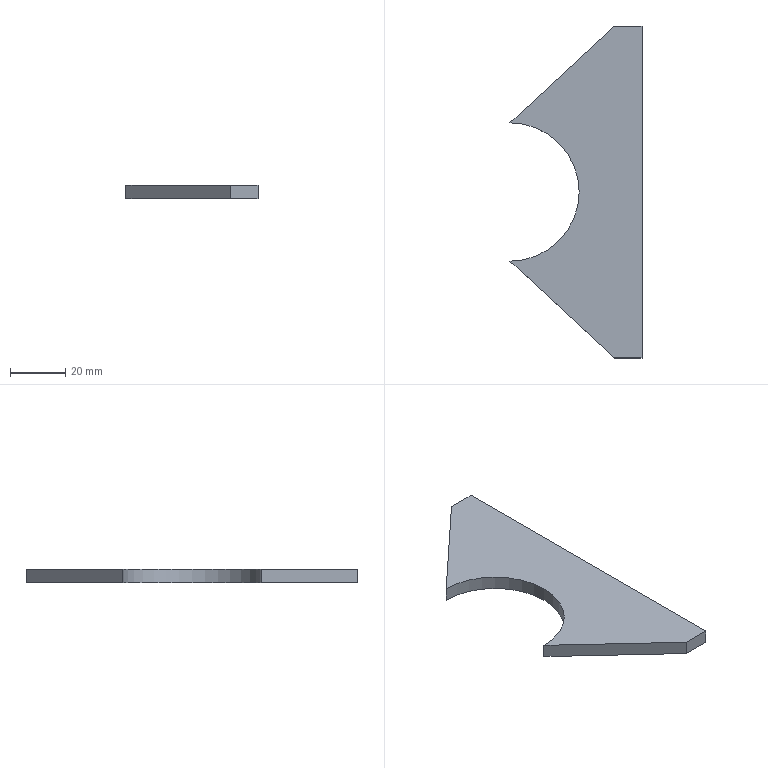Part | NX | 1 solid | 8 faces | box 47.73 x 120 x 5 mm | volume 17127 mm3 | plane 7 | cylinder 1 | commonest cylinder face diameters 50 x1
STEP:
#1=CARTESIAN_POINT('',(0.,-25.,0.));
#2=VERTEX_POINT('',#1);
#3=CARTESIAN_POINT('',(37.73,-60.,0.));
#4=VERTEX_POINT('',#3);
#5=CARTESIAN_POINT('',(0.,-25.,0.));
#6=DIRECTION('',(0.7331,-0.6801,0.));
#7=VECTOR('',#6,1.);
#8=LINE('',#5,#7);
#9=EDGE_CURVE('',#2,#4,#8,.T.);
#10=ORIENTED_EDGE('',*,*,#9,.T.);
#11=CARTESIAN_POINT('',(37.73,-60.,5.));
#12=VERTEX_POINT('',#11);
#13=CARTESIAN_POINT('',(37.73,-60.,5.));
#14=DIRECTION('',(0.,0.,-1.));
#15=VECTOR('',#14,1.);
#16=LINE('',#13,#15);
#17=EDGE_CURVE('',#12,#4,#16,.T.);
#18=ORIENTED_EDGE('',*,*,#17,.F.);
#19=CARTESIAN_POINT('',(0.,-25.,5.));
#20=VERTEX_POINT('',#19);
#21=CARTESIAN_POINT('',(0.,-25.,5.));
#22=DIRECTION('',(0.7331,-0.6801,0.));
#23=VECTOR('',#22,1.);
#24=LINE('',#21,#23);
#25=EDGE_CURVE('',#20,#12,#24,.T.);
#26=ORIENTED_EDGE('',*,*,#25,.F.);
#27=CARTESIAN_POINT('',(0.,-25.,5.));
#28=DIRECTION('',(0.,0.,-1.));
#29=VECTOR('',#28,1.);
#30=LINE('',#27,#29);
#31=EDGE_CURVE('',#20,#2,#30,.T.);
#32=ORIENTED_EDGE('',*,*,#31,.T.);
#33=EDGE_LOOP('',(#10,#18,#26,#32));
#34=FACE_OUTER_BOUND('',#33,.T.);
#35=CARTESIAN_POINT('',(0.,-25.,5.));
#36=DIRECTION('',(0.6801,0.7331,0.));
#37=DIRECTION('',(-0.7331,0.6801,0.));
#38=AXIS2_PLACEMENT_3D('',#35,#36,#37);
#39=PLANE('',#38);
#40=ADVANCED_FACE('',(#34),#39,.F.);
#41=CARTESIAN_POINT('',(47.73,-60.,0.));
#42=VERTEX_POINT('',#41);
#43=CARTESIAN_POINT('',(47.73,-60.,0.));
#44=DIRECTION('',(-1.,0.,0.));
#45=VECTOR('',#44,1.);
#46=LINE('',#43,#45);
#47=EDGE_CURVE('',#42,#4,#46,.T.);
#48=ORIENTED_EDGE('',*,*,#47,.F.);
#49=CARTESIAN_POINT('',(47.73,-60.,5.));
#50=VERTEX_POINT('',#49);
#51=CARTESIAN_POINT('',(47.73,-60.,5.));
#52=DIRECTION('',(0.,0.,-1.));
#53=VECTOR('',#52,1.);
#54=LINE('',#51,#53);
#55=EDGE_CURVE('',#50,#42,#54,.T.);
#56=ORIENTED_EDGE('',*,*,#55,.F.);
#57=CARTESIAN_POINT('',(47.73,-60.,5.));
#58=DIRECTION('',(-1.,0.,0.));
#59=VECTOR('',#58,1.);
#60=LINE('',#57,#59);
#61=EDGE_CURVE('',#50,#12,#60,.T.);
#62=ORIENTED_EDGE('',*,*,#61,.T.);
#63=ORIENTED_EDGE('',*,*,#17,.T.);
#64=EDGE_LOOP('',(#48,#56,#62,#63));
#65=FACE_OUTER_BOUND('',#64,.T.);
#66=CARTESIAN_POINT('',(47.73,-60.,5.));
#67=DIRECTION('',(0.,-1.,0.));
#68=DIRECTION('',(0.,0.,-1.));
#69=AXIS2_PLACEMENT_3D('',#66,#67,#68);
#70=PLANE('',#69);
#71=ADVANCED_FACE('',(#65),#70,.T.);
#72=CARTESIAN_POINT('',(47.73,60.,0.));
#73=VERTEX_POINT('',#72);
#74=CARTESIAN_POINT('',(47.73,0.,0.));
#75=DIRECTION('',(0.,1.,0.));
#76=VECTOR('',#75,1.);
#77=LINE('',#74,#76);
#78=EDGE_CURVE('',#42,#73,#77,.T.);
#79=ORIENTED_EDGE('',*,*,#78,.T.);
#80=CARTESIAN_POINT('',(47.73,60.,5.));
#81=VERTEX_POINT('',#80);
#82=CARTESIAN_POINT('',(47.73,60.,5.));
#83=DIRECTION('',(0.,0.,-1.));
#84=VECTOR('',#83,1.);
#85=LINE('',#82,#84);
#86=EDGE_CURVE('',#81,#73,#85,.T.);
#87=ORIENTED_EDGE('',*,*,#86,.F.);
#88=CARTESIAN_POINT('',(47.73,0.,5.));
#89=DIRECTION('',(0.,-1.,0.));
#90=VECTOR('',#89,1.);
#91=LINE('',#88,#90);
#92=EDGE_CURVE('',#81,#50,#91,.T.);
#93=ORIENTED_EDGE('',*,*,#92,.T.);
#94=ORIENTED_EDGE('',*,*,#55,.T.);
#95=EDGE_LOOP('',(#79,#87,#93,#94));
#96=FACE_OUTER_BOUND('',#95,.T.);
#97=CARTESIAN_POINT('',(47.73,0.,5.));
#98=DIRECTION('',(-1.,0.,0.));
#99=DIRECTION('',(0.,0.,1.));
#100=AXIS2_PLACEMENT_3D('',#97,#98,#99);
#101=PLANE('',#100);
#102=ADVANCED_FACE('',(#96),#101,.F.);
#103=CARTESIAN_POINT('',(37.73,60.,0.));
#104=VERTEX_POINT('',#103);
#105=CARTESIAN_POINT('',(47.73,60.,0.));
#106=DIRECTION('',(-1.,0.,0.));
#107=VECTOR('',#106,1.);
#108=LINE('',#105,#107);
#109=EDGE_CURVE('',#73,#104,#108,.T.);
#110=ORIENTED_EDGE('',*,*,#109,.T.);
#111=CARTESIAN_POINT('',(37.73,60.,5.));
#112=VERTEX_POINT('',#111);
#113=CARTESIAN_POINT('',(37.73,60.,5.));
#114=DIRECTION('',(0.,0.,-1.));
#115=VECTOR('',#114,1.);
#116=LINE('',#113,#115);
#117=EDGE_CURVE('',#112,#104,#116,.T.);
#118=ORIENTED_EDGE('',*,*,#117,.F.);
#119=CARTESIAN_POINT('',(47.73,60.,5.));
#120=DIRECTION('',(-1.,0.,0.));
#121=VECTOR('',#120,1.);
#122=LINE('',#119,#121);
#123=EDGE_CURVE('',#81,#112,#122,.T.);
#124=ORIENTED_EDGE('',*,*,#123,.F.);
#125=ORIENTED_EDGE('',*,*,#86,.T.);
#126=EDGE_LOOP('',(#110,#118,#124,#125));
#127=FACE_OUTER_BOUND('',#126,.T.);
#128=CARTESIAN_POINT('',(47.73,60.,5.));
#129=DIRECTION('',(0.,-1.,0.));
#130=DIRECTION('',(0.,0.,-1.));
#131=AXIS2_PLACEMENT_3D('',#128,#129,#130);
#132=PLANE('',#131);
#133=ADVANCED_FACE('',(#127),#132,.F.);
#134=CARTESIAN_POINT('',(0.,25.,0.));
#135=VERTEX_POINT('',#134);
#136=CARTESIAN_POINT('',(0.,25.,0.));
#137=DIRECTION('',(0.7331,0.6801,0.));
#138=VECTOR('',#137,1.);
#139=LINE('',#136,#138);
#140=EDGE_CURVE('',#135,#104,#139,.T.);
#141=ORIENTED_EDGE('',*,*,#140,.F.);
#142=CARTESIAN_POINT('',(0.,25.,5.));
#143=VERTEX_POINT('',#142);
#144=CARTESIAN_POINT('',(0.,25.,5.));
#145=DIRECTION('',(0.,0.,-1.));
#146=VECTOR('',#145,1.);
#147=LINE('',#144,#146);
#148=EDGE_CURVE('',#143,#135,#147,.T.);
#149=ORIENTED_EDGE('',*,*,#148,.F.);
#150=CARTESIAN_POINT('',(0.,25.,5.));
#151=DIRECTION('',(0.7331,0.6801,0.));
#152=VECTOR('',#151,1.);
#153=LINE('',#150,#152);
#154=EDGE_CURVE('',#143,#112,#153,.T.);
#155=ORIENTED_EDGE('',*,*,#154,.T.);
#156=ORIENTED_EDGE('',*,*,#117,.T.);
#157=EDGE_LOOP('',(#141,#149,#155,#156));
#158=FACE_OUTER_BOUND('',#157,.T.);
#159=CARTESIAN_POINT('',(0.,25.,5.));
#160=DIRECTION('',(-0.6801,0.7331,0.));
#161=DIRECTION('',(-0.7331,-0.6801,0.));
#162=AXIS2_PLACEMENT_3D('',#159,#160,#161);
#163=PLANE('',#162);
#164=ADVANCED_FACE('',(#158),#163,.T.);
#165=CARTESIAN_POINT('',(0.,0.,0.));
#166=DIRECTION('',(0.,0.,1.));
#167=DIRECTION('',(1.,0.,0.));
#168=AXIS2_PLACEMENT_3D('',#165,#166,#167);
#169=CIRCLE('',#168,25.);
#170=EDGE_CURVE('',#2,#135,#169,.T.);
#171=ORIENTED_EDGE('',*,*,#170,.F.);
#172=ORIENTED_EDGE('',*,*,#31,.F.);
#173=CARTESIAN_POINT('',(0.,0.,5.));
#174=DIRECTION('',(0.,0.,1.));
#175=DIRECTION('',(1.,0.,0.));
#176=AXIS2_PLACEMENT_3D('',#173,#174,#175);
#177=CIRCLE('',#176,25.);
#178=EDGE_CURVE('',#20,#143,#177,.T.);
#179=ORIENTED_EDGE('',*,*,#178,.T.);
#180=ORIENTED_EDGE('',*,*,#148,.T.);
#181=EDGE_LOOP('',(#171,#172,#179,#180));
#182=FACE_OUTER_BOUND('',#181,.T.);
#183=CARTESIAN_POINT('',(0.,0.,5.));
#184=DIRECTION('',(0.,0.,-1.));
#185=DIRECTION('',(-1.,0.,0.));
#186=AXIS2_PLACEMENT_3D('',#183,#184,#185);
#187=CYLINDRICAL_SURFACE('',#186,25.);
#188=ADVANCED_FACE('',(#182),#187,.F.);
#189=ORIENTED_EDGE('',*,*,#25,.T.);
#190=ORIENTED_EDGE('',*,*,#61,.F.);
#191=ORIENTED_EDGE('',*,*,#92,.F.);
#192=ORIENTED_EDGE('',*,*,#123,.T.);
#193=ORIENTED_EDGE('',*,*,#154,.F.);
#194=ORIENTED_EDGE('',*,*,#178,.F.);
#195=EDGE_LOOP('',(#189,#190,#191,#192,#193,#194));
#196=FACE_OUTER_BOUND('',#195,.T.);
#197=CARTESIAN_POINT('',(0.,0.,5.));
#198=DIRECTION('',(0.,0.,1.));
#199=DIRECTION('',(1.,0.,0.));
#200=AXIS2_PLACEMENT_3D('',#197,#198,#199);
#201=PLANE('',#200);
#202=ADVANCED_FACE('',(#196),#201,.T.);
#203=ORIENTED_EDGE('',*,*,#9,.F.);
#204=ORIENTED_EDGE('',*,*,#170,.T.);
#205=ORIENTED_EDGE('',*,*,#140,.T.);
#206=ORIENTED_EDGE('',*,*,#109,.F.);
#207=ORIENTED_EDGE('',*,*,#78,.F.);
#208=ORIENTED_EDGE('',*,*,#47,.T.);
#209=EDGE_LOOP('',(#203,#204,#205,#206,#207,#208));
#210=FACE_OUTER_BOUND('',#209,.T.);
#211=CARTESIAN_POINT('',(0.,0.,0.));
#212=DIRECTION('',(0.,0.,1.));
#213=DIRECTION('',(1.,0.,0.));
#214=AXIS2_PLACEMENT_3D('',#211,#212,#213);
#215=PLANE('',#214);
#216=ADVANCED_FACE('',(#210),#215,.F.);
#217=CLOSED_SHELL('',(#40,#71,#102,#133,#164,#188,#202,#216));
#218=MANIFOLD_SOLID_BREP('',#217);
#219=(LENGTH_UNIT()NAMED_UNIT(*)SI_UNIT(.MILLI.,.METRE.));
#220=UNCERTAINTY_MEASURE_WITH_UNIT(LENGTH_MEASURE(0.00002),#219,'','');
#221=(NAMED_UNIT(*)PLANE_ANGLE_UNIT()SI_UNIT($,.RADIAN.));
#222=PLANE_ANGLE_MEASURE_WITH_UNIT(PLANE_ANGLE_MEASURE(0.01745),#221);
#223=DIMENSIONAL_EXPONENTS(0.,0.,0.,0.,0.,0.,0.);
#224=(CONVERSION_BASED_UNIT('DEGREE',#222)NAMED_UNIT(#223)PLANE_ANGLE_UNIT());
#225=(NAMED_UNIT(*)SI_UNIT($,.STERADIAN.)SOLID_ANGLE_UNIT());
#226=(GEOMETRIC_REPRESENTATION_CONTEXT(3)GLOBAL_UNCERTAINTY_ASSIGNED_CONTEXT((#220))GLOBAL_UNIT_ASSIGNED_CONTEXT((#219,#224,#225))REPRESENTATION_CONTEXT('',''));
#227=ADVANCED_BREP_SHAPE_REPRESENTATION('',(#218),#226);